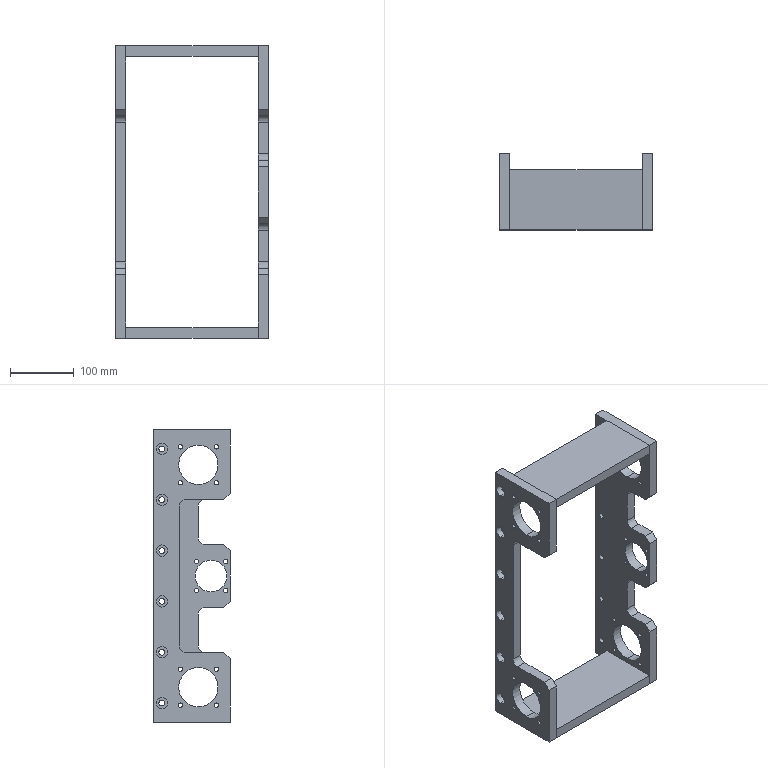Part | SolidWorks | features ICE 7, HoleWzd 3, Chamfer 2, Fillet 2, MirrorPattern 2, Extrusion 1 | 4 solids | 158 faces | box 240 x 120 x 460 mm | volume 1705402 mm3 | cylinder 104 | plane 54 | commonest cylinder face diameters 6.8 x40 9 x24 18 x24 62 x8 20 x6 50 x2